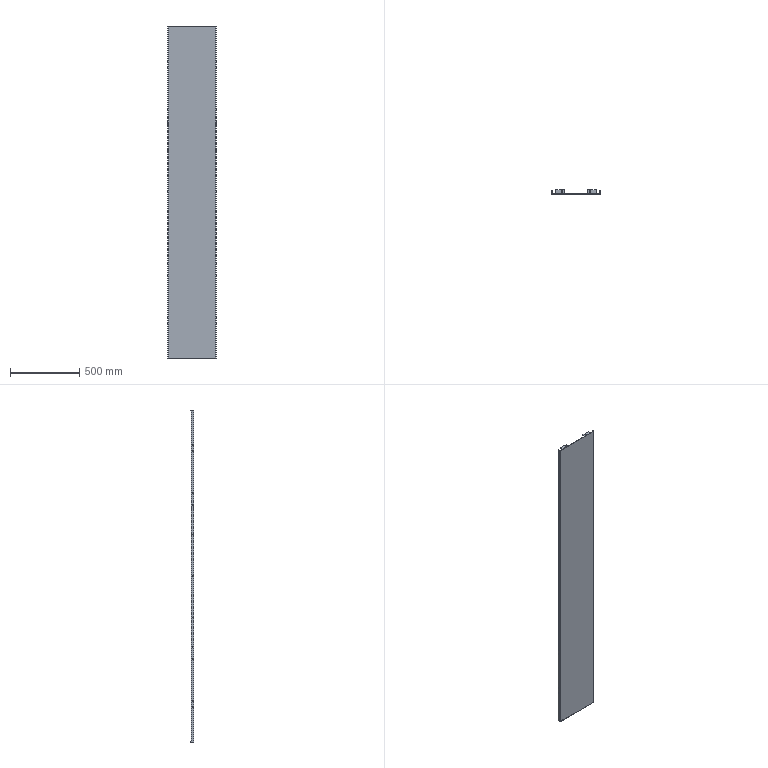Part | SolidWorks | features ICE 5, FlatPattern 1, SMBaseFlange 1, SheetMetal 1 | 1 solid | 98 faces | box 350 x 25 x 2396 mm | volume 1834620 mm3 | cylinder 56 | plane 42 | commonest cylinder face diameters 6.2 x44 7 x8 0.4 x2 4.4 x2